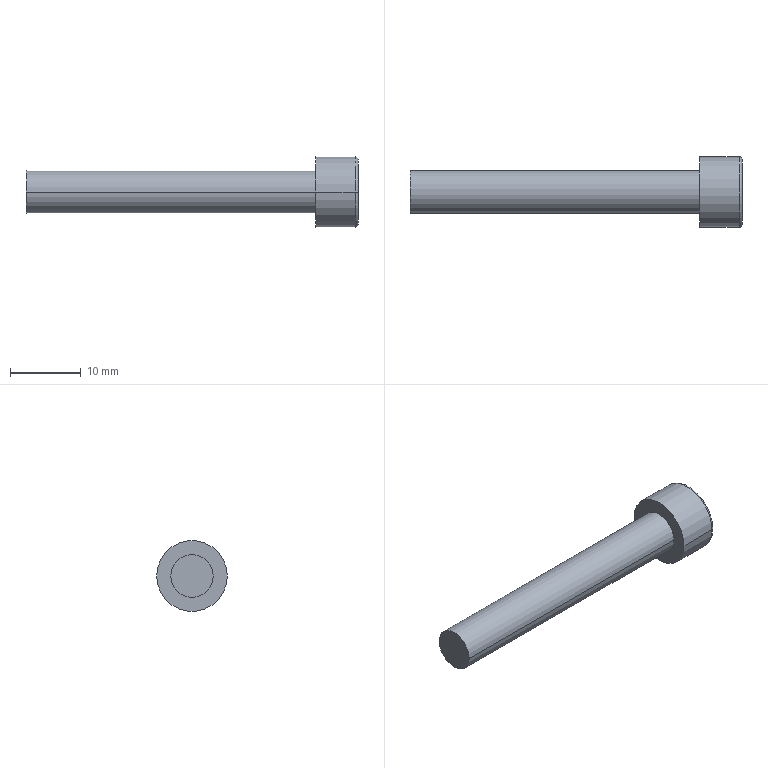Part | STEP file | 4-20.sldasm-Part-4 | 1 solid | 16 faces | box 47 x 10 x 10 mm | volume 1564 mm3 | plane 10 | cylinder 4 | torus 2 | commonest cylinder face diameters 6 x2 10 x2
STEP:
#1=CARTESIAN_POINT('',(251.,437.,208.));
#2=VERTEX_POINT('',#1);
#3=CARTESIAN_POINT('',(251.,447.,208.));
#4=VERTEX_POINT('',#3);
#5=CARTESIAN_POINT('',(251.,442.,208.));
#6=DIRECTION('',(1.,0.,0.));
#7=DIRECTION('',(0.,-1.,0.));
#8=AXIS2_PLACEMENT_3D('',#5,#6,#7);
#9=CIRCLE('',#8,5.);
#10=EDGE_CURVE('',#2,#4,#9,.T.);
#11=ORIENTED_EDGE('',*,*,#10,.T.);
#12=CARTESIAN_POINT('',(256.6,447.,208.));
#13=VERTEX_POINT('',#12);
#14=CARTESIAN_POINT('',(258.675,447.,208.));
#15=DIRECTION('',(1.,0.,0.));
#16=VECTOR('',#15,1000.);
#17=LINE('',#14,#16);
#18=EDGE_CURVE('',#4,#13,#17,.T.);
#19=ORIENTED_EDGE('',*,*,#18,.T.);
#20=CARTESIAN_POINT('',(256.6,437.,208.));
#21=VERTEX_POINT('',#20);
#22=CARTESIAN_POINT('',(256.6,442.,208.));
#23=DIRECTION('',(1.,0.,0.));
#24=DIRECTION('',(0.,-1.,0.));
#25=AXIS2_PLACEMENT_3D('',#22,#23,#24);
#26=CIRCLE('',#25,5.);
#27=EDGE_CURVE('',#21,#13,#26,.T.);
#28=ORIENTED_EDGE('',*,*,#27,.F.);
#29=CARTESIAN_POINT('',(258.675,437.,208.));
#30=DIRECTION('',(1.,0.,0.));
#31=VECTOR('',#30,1000.);
#32=LINE('',#29,#31);
#33=EDGE_CURVE('',#2,#21,#32,.T.);
#34=ORIENTED_EDGE('',*,*,#33,.F.);
#35=EDGE_LOOP('',(#11,#19,#28,#34));
#36=FACE_OUTER_BOUND('',#35,.T.);
#37=CARTESIAN_POINT('',(258.675,442.,208.));
#38=DIRECTION('',(1.,0.,0.));
#39=DIRECTION('',(0.,-1.,0.));
#40=AXIS2_PLACEMENT_3D('',#37,#38,#39);
#41=CYLINDRICAL_SURFACE('',#40,5.);
#42=ADVANCED_FACE('',(#36),#41,.T.);
#43=ORIENTED_EDGE('',*,*,#27,.T.);
#44=CARTESIAN_POINT('',(257.,446.6,208.));
#45=VERTEX_POINT('',#44);
#46=CARTESIAN_POINT('',(256.6,446.6,208.));
#47=DIRECTION('',(0.,0.,-1.));
#48=DIRECTION('',(-1.,0.,0.));
#49=AXIS2_PLACEMENT_3D('',#46,#47,#48);
#50=CIRCLE('',#49,0.4);
#51=EDGE_CURVE('',#13,#45,#50,.T.);
#52=ORIENTED_EDGE('',*,*,#51,.T.);
#53=CARTESIAN_POINT('',(257.,437.4,208.));
#54=VERTEX_POINT('',#53);
#55=CARTESIAN_POINT('',(257.,442.,208.));
#56=DIRECTION('',(1.,0.,0.));
#57=DIRECTION('',(0.,-1.,0.));
#58=AXIS2_PLACEMENT_3D('',#55,#56,#57);
#59=CIRCLE('',#58,4.6);
#60=EDGE_CURVE('',#54,#45,#59,.T.);
#61=ORIENTED_EDGE('',*,*,#60,.F.);
#62=CARTESIAN_POINT('',(256.6,437.4,208.));
#63=DIRECTION('',(0.,0.,1.));
#64=DIRECTION('',(1.,0.,0.));
#65=AXIS2_PLACEMENT_3D('',#62,#63,#64);
#66=CIRCLE('',#65,0.4);
#67=EDGE_CURVE('',#21,#54,#66,.T.);
#68=ORIENTED_EDGE('',*,*,#67,.F.);
#69=EDGE_LOOP('',(#43,#52,#61,#68));
#70=FACE_OUTER_BOUND('',#69,.T.);
#71=CARTESIAN_POINT('',(256.6,442.,208.));
#72=DIRECTION('',(1.,0.,0.));
#73=DIRECTION('',(0.,-1.,0.));
#74=AXIS2_PLACEMENT_3D('',#71,#72,#73);
#75=TOROIDAL_SURFACE('',#74,4.6,0.4);
#76=ADVANCED_FACE('',(#70),#75,.T.);
#77=CARTESIAN_POINT('',(210.,439.,208.));
#78=VERTEX_POINT('',#77);
#79=CARTESIAN_POINT('',(210.,445.,208.));
#80=VERTEX_POINT('',#79);
#81=CARTESIAN_POINT('',(210.,442.,208.));
#82=DIRECTION('',(1.,0.,0.));
#83=DIRECTION('',(0.,-1.,0.));
#84=AXIS2_PLACEMENT_3D('',#81,#82,#83);
#85=CIRCLE('',#84,3.);
#86=EDGE_CURVE('',#78,#80,#85,.T.);
#87=ORIENTED_EDGE('',*,*,#86,.T.);
#88=CARTESIAN_POINT('',(251.,445.,208.));
#89=VERTEX_POINT('',#88);
#90=CARTESIAN_POINT('',(258.675,445.,208.));
#91=DIRECTION('',(1.,0.,0.));
#92=VECTOR('',#91,1000.);
#93=LINE('',#90,#92);
#94=EDGE_CURVE('',#80,#89,#93,.T.);
#95=ORIENTED_EDGE('',*,*,#94,.T.);
#96=CARTESIAN_POINT('',(251.,439.,208.));
#97=VERTEX_POINT('',#96);
#98=CARTESIAN_POINT('',(251.,442.,208.));
#99=DIRECTION('',(1.,0.,0.));
#100=DIRECTION('',(0.,-1.,0.));
#101=AXIS2_PLACEMENT_3D('',#98,#99,#100);
#102=CIRCLE('',#101,3.);
#103=EDGE_CURVE('',#97,#89,#102,.T.);
#104=ORIENTED_EDGE('',*,*,#103,.F.);
#105=CARTESIAN_POINT('',(258.675,439.,208.));
#106=DIRECTION('',(1.,0.,0.));
#107=VECTOR('',#106,1000.);
#108=LINE('',#105,#107);
#109=EDGE_CURVE('',#78,#97,#108,.T.);
#110=ORIENTED_EDGE('',*,*,#109,.F.);
#111=EDGE_LOOP('',(#87,#95,#104,#110));
#112=FACE_OUTER_BOUND('',#111,.T.);
#113=CARTESIAN_POINT('',(258.675,442.,208.));
#114=DIRECTION('',(1.,0.,0.));
#115=DIRECTION('',(0.,-1.,0.));
#116=AXIS2_PLACEMENT_3D('',#113,#114,#115);
#117=CYLINDRICAL_SURFACE('',#116,3.);
#118=ADVANCED_FACE('',(#112),#117,.T.);
#119=ORIENTED_EDGE('',*,*,#94,.F.);
#120=CARTESIAN_POINT('',(210.,442.,208.));
#121=DIRECTION('',(1.,0.,0.));
#122=DIRECTION('',(0.,-1.,0.));
#123=AXIS2_PLACEMENT_3D('',#120,#121,#122);
#124=CIRCLE('',#123,3.);
#125=EDGE_CURVE('',#80,#78,#124,.T.);
#126=ORIENTED_EDGE('',*,*,#125,.T.);
#127=ORIENTED_EDGE('',*,*,#109,.T.);
#128=CARTESIAN_POINT('',(251.,442.,208.));
#129=DIRECTION('',(1.,0.,0.));
#130=DIRECTION('',(0.,-1.,0.));
#131=AXIS2_PLACEMENT_3D('',#128,#129,#130);
#132=CIRCLE('',#131,3.);
#133=EDGE_CURVE('',#89,#97,#132,.T.);
#134=ORIENTED_EDGE('',*,*,#133,.F.);
#135=EDGE_LOOP('',(#119,#126,#127,#134));
#136=FACE_OUTER_BOUND('',#135,.T.);
#137=CARTESIAN_POINT('',(258.675,442.,208.));
#138=DIRECTION('',(1.,0.,0.));
#139=DIRECTION('',(0.,-1.,0.));
#140=AXIS2_PLACEMENT_3D('',#137,#138,#139);
#141=CYLINDRICAL_SURFACE('',#140,3.);
#142=ADVANCED_FACE('',(#136),#141,.T.);
#143=CARTESIAN_POINT('',(257.,439.5,206.557));
#144=VERTEX_POINT('',#143);
#145=CARTESIAN_POINT('',(257.,442.,205.113));
#146=VERTEX_POINT('',#145);
#147=CARTESIAN_POINT('',(257.,439.5,206.557));
#148=DIRECTION('',(0.,0.866,-0.5));
#149=VECTOR('',#148,1000.);
#150=LINE('',#147,#149);
#151=EDGE_CURVE('',#144,#146,#150,.T.);
#152=ORIENTED_EDGE('',*,*,#151,.F.);
#153=CARTESIAN_POINT('',(257.,439.5,209.443));
#154=VERTEX_POINT('',#153);
#155=CARTESIAN_POINT('',(257.,439.5,209.443));
#156=DIRECTION('',(0.,0.,-1.));
#157=VECTOR('',#156,1000.);
#158=LINE('',#155,#157);
#159=EDGE_CURVE('',#154,#144,#158,.T.);
#160=ORIENTED_EDGE('',*,*,#159,.F.);
#161=CARTESIAN_POINT('',(257.,442.,210.887));
#162=VERTEX_POINT('',#161);
#163=CARTESIAN_POINT('',(257.,442.,210.887));
#164=DIRECTION('',(0.,-0.866,-0.5));
#165=VECTOR('',#164,1000.);
#166=LINE('',#163,#165);
#167=EDGE_CURVE('',#162,#154,#166,.T.);
#168=ORIENTED_EDGE('',*,*,#167,.F.);
#169=CARTESIAN_POINT('',(257.,444.5,209.443));
#170=VERTEX_POINT('',#169);
#171=CARTESIAN_POINT('',(257.,444.5,209.443));
#172=DIRECTION('',(0.,-0.866,0.5));
#173=VECTOR('',#172,1000.);
#174=LINE('',#171,#173);
#175=EDGE_CURVE('',#170,#162,#174,.T.);
#176=ORIENTED_EDGE('',*,*,#175,.F.);
#177=CARTESIAN_POINT('',(257.,444.5,206.557));
#178=VERTEX_POINT('',#177);
#179=CARTESIAN_POINT('',(257.,444.5,206.557));
#180=DIRECTION('',(0.,0.,1.));
#181=VECTOR('',#180,1000.);
#182=LINE('',#179,#181);
#183=EDGE_CURVE('',#178,#170,#182,.T.);
#184=ORIENTED_EDGE('',*,*,#183,.F.);
#185=CARTESIAN_POINT('',(257.,442.,205.113));
#186=DIRECTION('',(0.,0.866,0.5));
#187=VECTOR('',#186,1000.);
#188=LINE('',#185,#187);
#189=EDGE_CURVE('',#146,#178,#188,.T.);
#190=ORIENTED_EDGE('',*,*,#189,.F.);
#191=EDGE_LOOP('',(#152,#160,#168,#176,#184,#190));
#192=FACE_BOUND('',#191,.T.);
#193=ORIENTED_EDGE('',*,*,#60,.T.);
#194=CARTESIAN_POINT('',(257.,442.,208.));
#195=DIRECTION('',(1.,0.,0.));
#196=DIRECTION('',(0.,-1.,0.));
#197=AXIS2_PLACEMENT_3D('',#194,#195,#196);
#198=CIRCLE('',#197,4.6);
#199=EDGE_CURVE('',#45,#54,#198,.T.);
#200=ORIENTED_EDGE('',*,*,#199,.T.);
#201=EDGE_LOOP('',(#193,#200));
#202=FACE_OUTER_BOUND('',#201,.T.);
#203=CARTESIAN_POINT('',(257.,442.,208.));
#204=DIRECTION('',(1.,0.,0.));
#205=DIRECTION('',(0.,-1.,0.));
#206=AXIS2_PLACEMENT_3D('',#203,#204,#205);
#207=PLANE('',#206);
#208=ADVANCED_FACE('',(#192,#202),#207,.T.);
#209=ORIENTED_EDGE('',*,*,#51,.F.);
#210=CARTESIAN_POINT('',(256.6,442.,208.));
#211=DIRECTION('',(1.,0.,0.));
#212=DIRECTION('',(0.,-1.,0.));
#213=AXIS2_PLACEMENT_3D('',#210,#211,#212);
#214=CIRCLE('',#213,5.);
#215=EDGE_CURVE('',#13,#21,#214,.T.);
#216=ORIENTED_EDGE('',*,*,#215,.T.);
#217=ORIENTED_EDGE('',*,*,#67,.T.);
#218=ORIENTED_EDGE('',*,*,#199,.F.);
#219=EDGE_LOOP('',(#209,#216,#217,#218));
#220=FACE_OUTER_BOUND('',#219,.T.);
#221=CARTESIAN_POINT('',(256.6,442.,208.));
#222=DIRECTION('',(1.,0.,0.));
#223=DIRECTION('',(0.,-1.,0.));
#224=AXIS2_PLACEMENT_3D('',#221,#222,#223);
#225=TOROIDAL_SURFACE('',#224,4.6,0.4);
#226=ADVANCED_FACE('',(#220),#225,.T.);
#227=ORIENTED_EDGE('',*,*,#18,.F.);
#228=CARTESIAN_POINT('',(251.,442.,208.));
#229=DIRECTION('',(1.,0.,0.));
#230=DIRECTION('',(0.,-1.,0.));
#231=AXIS2_PLACEMENT_3D('',#228,#229,#230);
#232=CIRCLE('',#231,5.);
#233=EDGE_CURVE('',#4,#2,#232,.T.);
#234=ORIENTED_EDGE('',*,*,#233,.T.);
#235=ORIENTED_EDGE('',*,*,#33,.T.);
#236=ORIENTED_EDGE('',*,*,#215,.F.);
#237=EDGE_LOOP('',(#227,#234,#235,#236));
#238=FACE_OUTER_BOUND('',#237,.T.);
#239=CARTESIAN_POINT('',(258.675,442.,208.));
#240=DIRECTION('',(1.,0.,0.));
#241=DIRECTION('',(0.,-1.,0.));
#242=AXIS2_PLACEMENT_3D('',#239,#240,#241);
#243=CYLINDRICAL_SURFACE('',#242,5.);
#244=ADVANCED_FACE('',(#238),#243,.T.);
#245=ORIENTED_EDGE('',*,*,#103,.T.);
#246=ORIENTED_EDGE('',*,*,#133,.T.);
#247=EDGE_LOOP('',(#245,#246));
#248=FACE_BOUND('',#247,.T.);
#249=ORIENTED_EDGE('',*,*,#10,.F.);
#250=ORIENTED_EDGE('',*,*,#233,.F.);
#251=EDGE_LOOP('',(#249,#250));
#252=FACE_OUTER_BOUND('',#251,.T.);
#253=CARTESIAN_POINT('',(251.,442.,203.));
#254=DIRECTION('',(-1.,0.,0.));
#255=DIRECTION('',(0.,1.,0.));
#256=AXIS2_PLACEMENT_3D('',#253,#254,#255);
#257=PLANE('',#256);
#258=ADVANCED_FACE('',(#248,#252),#257,.T.);
#259=ORIENTED_EDGE('',*,*,#151,.T.);
#260=CARTESIAN_POINT('',(254.,442.,205.113));
#261=VERTEX_POINT('',#260);
#262=CARTESIAN_POINT('',(254.,442.,205.113));
#263=DIRECTION('',(1.,0.,0.));
#264=VECTOR('',#263,1000.);
#265=LINE('',#262,#264);
#266=EDGE_CURVE('',#261,#146,#265,.T.);
#267=ORIENTED_EDGE('',*,*,#266,.F.);
#268=CARTESIAN_POINT('',(254.,439.5,206.557));
#269=VERTEX_POINT('',#268);
#270=CARTESIAN_POINT('',(254.,439.5,206.557));
#271=DIRECTION('',(0.,0.866,-0.5));
#272=VECTOR('',#271,1000.);
#273=LINE('',#270,#272);
#274=EDGE_CURVE('',#269,#261,#273,.T.);
#275=ORIENTED_EDGE('',*,*,#274,.F.);
#276=CARTESIAN_POINT('',(254.,439.5,206.557));
#277=DIRECTION('',(1.,0.,0.));
#278=VECTOR('',#277,1000.);
#279=LINE('',#276,#278);
#280=EDGE_CURVE('',#269,#144,#279,.T.);
#281=ORIENTED_EDGE('',*,*,#280,.T.);
#282=EDGE_LOOP('',(#259,#267,#275,#281));
#283=FACE_OUTER_BOUND('',#282,.T.);
#284=CARTESIAN_POINT('',(254.,439.5,206.557));
#285=DIRECTION('',(0.,-0.5,-0.866));
#286=DIRECTION('',(0.,-0.866,0.5));
#287=AXIS2_PLACEMENT_3D('',#284,#285,#286);
#288=PLANE('',#287);
#289=ADVANCED_FACE('',(#283),#288,.F.);
#290=ORIENTED_EDGE('',*,*,#159,.T.);
#291=ORIENTED_EDGE('',*,*,#280,.F.);
#292=CARTESIAN_POINT('',(254.,439.5,209.443));
#293=VERTEX_POINT('',#292);
#294=CARTESIAN_POINT('',(254.,439.5,209.443));
#295=DIRECTION('',(0.,0.,-1.));
#296=VECTOR('',#295,1000.);
#297=LINE('',#294,#296);
#298=EDGE_CURVE('',#293,#269,#297,.T.);
#299=ORIENTED_EDGE('',*,*,#298,.F.);
#300=CARTESIAN_POINT('',(254.,439.5,209.443));
#301=DIRECTION('',(1.,0.,0.));
#302=VECTOR('',#301,1000.);
#303=LINE('',#300,#302);
#304=EDGE_CURVE('',#293,#154,#303,.T.);
#305=ORIENTED_EDGE('',*,*,#304,.T.);
#306=EDGE_LOOP('',(#290,#291,#299,#305));
#307=FACE_OUTER_BOUND('',#306,.T.);
#308=CARTESIAN_POINT('',(254.,439.5,209.443));
#309=DIRECTION('',(0.,-1.,0.));
#310=DIRECTION('',(-1.,0.,0.));
#311=AXIS2_PLACEMENT_3D('',#308,#309,#310);
#312=PLANE('',#311);
#313=ADVANCED_FACE('',(#307),#312,.F.);
#314=ORIENTED_EDGE('',*,*,#167,.T.);
#315=ORIENTED_EDGE('',*,*,#304,.F.);
#316=CARTESIAN_POINT('',(254.,442.,210.887));
#317=VERTEX_POINT('',#316);
#318=CARTESIAN_POINT('',(254.,442.,210.887));
#319=DIRECTION('',(0.,-0.866,-0.5));
#320=VECTOR('',#319,1000.);
#321=LINE('',#318,#320);
#322=EDGE_CURVE('',#317,#293,#321,.T.);
#323=ORIENTED_EDGE('',*,*,#322,.F.);
#324=CARTESIAN_POINT('',(254.,442.,210.887));
#325=DIRECTION('',(1.,0.,0.));
#326=VECTOR('',#325,1000.);
#327=LINE('',#324,#326);
#328=EDGE_CURVE('',#317,#162,#327,.T.);
#329=ORIENTED_EDGE('',*,*,#328,.T.);
#330=EDGE_LOOP('',(#314,#315,#323,#329));
#331=FACE_OUTER_BOUND('',#330,.T.);
#332=CARTESIAN_POINT('',(254.,442.,210.887));
#333=DIRECTION('',(0.,-0.5,0.866));
#334=DIRECTION('',(0.,0.866,0.5));
#335=AXIS2_PLACEMENT_3D('',#332,#333,#334);
#336=PLANE('',#335);
#337=ADVANCED_FACE('',(#331),#336,.F.);
#338=ORIENTED_EDGE('',*,*,#175,.T.);
#339=ORIENTED_EDGE('',*,*,#328,.F.);
#340=CARTESIAN_POINT('',(254.,444.5,209.443));
#341=VERTEX_POINT('',#340);
#342=CARTESIAN_POINT('',(254.,444.5,209.443));
#343=DIRECTION('',(0.,-0.866,0.5));
#344=VECTOR('',#343,1000.);
#345=LINE('',#342,#344);
#346=EDGE_CURVE('',#341,#317,#345,.T.);
#347=ORIENTED_EDGE('',*,*,#346,.F.);
#348=CARTESIAN_POINT('',(254.,444.5,209.443));
#349=DIRECTION('',(1.,0.,0.));
#350=VECTOR('',#349,1000.);
#351=LINE('',#348,#350);
#352=EDGE_CURVE('',#341,#170,#351,.T.);
#353=ORIENTED_EDGE('',*,*,#352,.T.);
#354=EDGE_LOOP('',(#338,#339,#347,#353));
#355=FACE_OUTER_BOUND('',#354,.T.);
#356=CARTESIAN_POINT('',(254.,444.5,209.443));
#357=DIRECTION('',(0.,0.5,0.866));
#358=DIRECTION('',(0.,0.866,-0.5));
#359=AXIS2_PLACEMENT_3D('',#356,#357,#358);
#360=PLANE('',#359);
#361=ADVANCED_FACE('',(#355),#360,.F.);
#362=ORIENTED_EDGE('',*,*,#183,.T.);
#363=ORIENTED_EDGE('',*,*,#352,.F.);
#364=CARTESIAN_POINT('',(254.,444.5,206.557));
#365=VERTEX_POINT('',#364);
#366=CARTESIAN_POINT('',(254.,444.5,206.557));
#367=DIRECTION('',(0.,0.,1.));
#368=VECTOR('',#367,1000.);
#369=LINE('',#366,#368);
#370=EDGE_CURVE('',#365,#341,#369,.T.);
#371=ORIENTED_EDGE('',*,*,#370,.F.);
#372=CARTESIAN_POINT('',(254.,444.5,206.557));
#373=DIRECTION('',(1.,0.,0.));
#374=VECTOR('',#373,1000.);
#375=LINE('',#372,#374);
#376=EDGE_CURVE('',#365,#178,#375,.T.);
#377=ORIENTED_EDGE('',*,*,#376,.T.);
#378=EDGE_LOOP('',(#362,#363,#371,#377));
#379=FACE_OUTER_BOUND('',#378,.T.);
#380=CARTESIAN_POINT('',(254.,444.5,206.557));
#381=DIRECTION('',(0.,1.,0.));
#382=DIRECTION('',(0.,0.,-1.));
#383=AXIS2_PLACEMENT_3D('',#380,#381,#382);
#384=PLANE('',#383);
#385=ADVANCED_FACE('',(#379),#384,.F.);
#386=ORIENTED_EDGE('',*,*,#189,.T.);
#387=ORIENTED_EDGE('',*,*,#376,.F.);
#388=CARTESIAN_POINT('',(254.,442.,205.113));
#389=DIRECTION('',(0.,0.866,0.5));
#390=VECTOR('',#389,1000.);
#391=LINE('',#388,#390);
#392=EDGE_CURVE('',#261,#365,#391,.T.);
#393=ORIENTED_EDGE('',*,*,#392,.F.);
#394=ORIENTED_EDGE('',*,*,#266,.T.);
#395=EDGE_LOOP('',(#386,#387,#393,#394));
#396=FACE_OUTER_BOUND('',#395,.T.);
#397=CARTESIAN_POINT('',(254.,442.,205.113));
#398=DIRECTION('',(0.,0.5,-0.866));
#399=DIRECTION('',(0.,-0.866,-0.5));
#400=AXIS2_PLACEMENT_3D('',#397,#398,#399);
#401=PLANE('',#400);
#402=ADVANCED_FACE('',(#396),#401,.F.);
#403=ORIENTED_EDGE('',*,*,#274,.T.);
#404=ORIENTED_EDGE('',*,*,#392,.T.);
#405=ORIENTED_EDGE('',*,*,#370,.T.);
#406=ORIENTED_EDGE('',*,*,#346,.T.);
#407=ORIENTED_EDGE('',*,*,#322,.T.);
#408=ORIENTED_EDGE('',*,*,#298,.T.);
#409=EDGE_LOOP('',(#403,#404,#405,#406,#407,#408));
#410=FACE_OUTER_BOUND('',#409,.T.);
#411=CARTESIAN_POINT('',(254.,442.,205.113));
#412=DIRECTION('',(1.,0.,0.));
#413=DIRECTION('',(0.,-1.,0.));
#414=AXIS2_PLACEMENT_3D('',#411,#412,#413);
#415=PLANE('',#414);
#416=ADVANCED_FACE('',(#410),#415,.T.);
#417=ORIENTED_EDGE('',*,*,#86,.F.);
#418=ORIENTED_EDGE('',*,*,#125,.F.);
#419=EDGE_LOOP('',(#417,#418));
#420=FACE_OUTER_BOUND('',#419,.T.);
#421=CARTESIAN_POINT('',(210.,328.,144.));
#422=DIRECTION('',(-1.,0.,0.));
#423=DIRECTION('',(0.,-1.,0.));
#424=AXIS2_PLACEMENT_3D('',#421,#422,#423);
#425=PLANE('',#424);
#426=ADVANCED_FACE('',(#420),#425,.T.);
#427=CLOSED_SHELL('',(#42,#76,#118,#142,#208,#226,#244,#258,#289,#313,#337,#361,#385,#402,#416,#426));
#428=MANIFOLD_SOLID_BREP('',#427);
#429=CARTESIAN_POINT('',(0.,0.,0.));
#430=DIRECTION('',(0.,0.,1.));
#431=DIRECTION('',(1.,0.,0.));
#432=AXIS2_PLACEMENT_3D('',#429,#430,#431);
#433=(LENGTH_UNIT()NAMED_UNIT(*)SI_UNIT(.MILLI.,.METRE.));
#434=UNCERTAINTY_MEASURE_WITH_UNIT(LENGTH_MEASURE(0.00001),#433,'','');
#435=(NAMED_UNIT(*)PLANE_ANGLE_UNIT()SI_UNIT($,.RADIAN.));
#436=(NAMED_UNIT(*)SI_UNIT($,.STERADIAN.)SOLID_ANGLE_UNIT());
#437=(GEOMETRIC_REPRESENTATION_CONTEXT(3)GLOBAL_UNCERTAINTY_ASSIGNED_CONTEXT((#434))GLOBAL_UNIT_ASSIGNED_CONTEXT((#433,#435,#436))REPRESENTATION_CONTEXT('',''));
#438=ADVANCED_BREP_SHAPE_REPRESENTATION('',(#428,#432),#437);